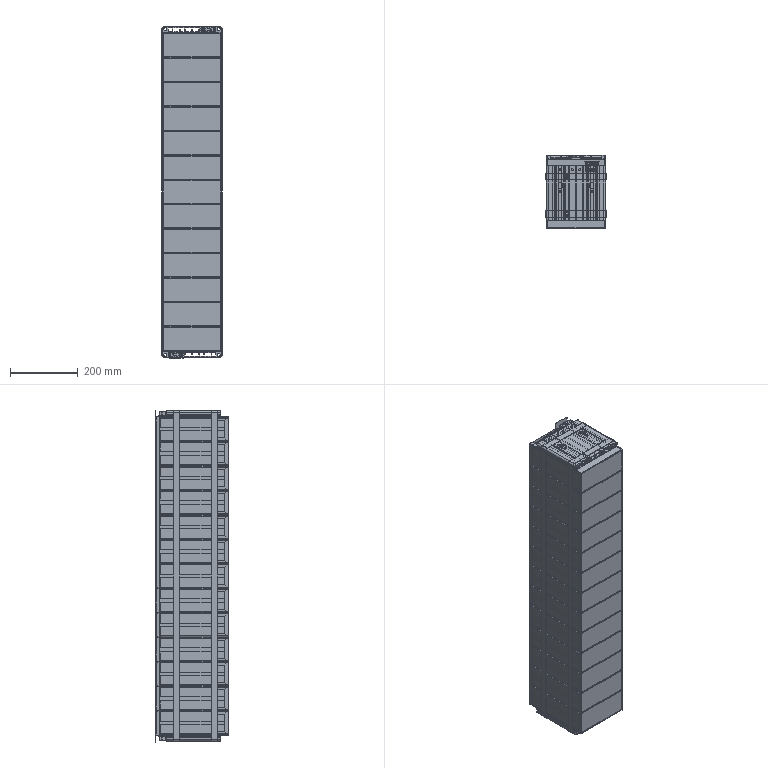Part | NX | features BREP 16 | 75 solids | 12833 faces | volume 34754714 mm3 | plane 7788 | cylinder 4716 | cone 159 | torus 82 | spline 60 | sphere 28 | commonest cylinder face diameters 8 x1000 2 x605 6 x440 4 x408 0.4 x236 3 x208